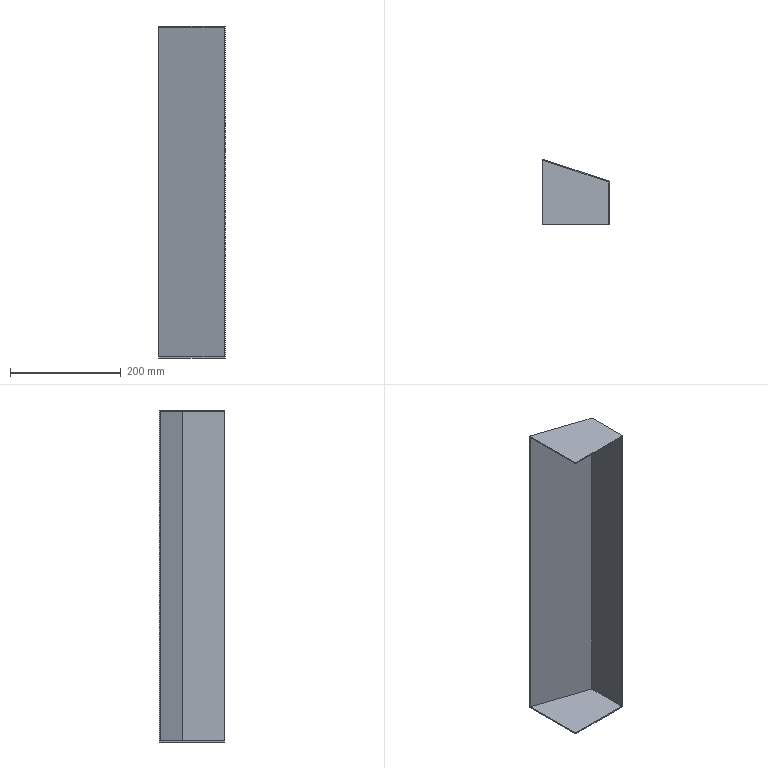Part | SolidWorks | features Extrusion 1, ICE 1, Shell 1 | 1 solid | 10 faces | box 120 x 118 x 600 mm | volume 288678 mm3 | plane 10
STEP:
#1=CARTESIAN_POINT('',(0.,120.,-300.));
#2=VERTEX_POINT('',#1);
#3=CARTESIAN_POINT('',(0.,2.,-300.));
#4=VERTEX_POINT('',#3);
#5=CARTESIAN_POINT('',(0.,0.,-300.));
#6=DIRECTION('',(0.,-1.,0.));
#7=VECTOR('',#6,1000.);
#8=LINE('',#5,#7);
#9=EDGE_CURVE('',#2,#4,#8,.T.);
#10=ORIENTED_EDGE('',*,*,#9,.T.);
#11=CARTESIAN_POINT('',(0.,2.,-298.));
#12=VERTEX_POINT('',#11);
#13=CARTESIAN_POINT('',(0.,2.,300.));
#14=DIRECTION('',(0.,0.,-1.));
#15=VECTOR('',#14,1000.);
#16=LINE('',#13,#15);
#17=EDGE_CURVE('',#12,#4,#16,.T.);
#18=ORIENTED_EDGE('',*,*,#17,.F.);
#19=CARTESIAN_POINT('',(0.,117.892,-298.));
#20=VERTEX_POINT('',#19);
#21=CARTESIAN_POINT('',(0.,0.,-298.));
#22=DIRECTION('',(0.,-1.,0.));
#23=VECTOR('',#22,1000.);
#24=LINE('',#21,#23);
#25=EDGE_CURVE('',#20,#12,#24,.T.);
#26=ORIENTED_EDGE('',*,*,#25,.F.);
#27=CARTESIAN_POINT('',(0.,117.892,298.));
#28=VERTEX_POINT('',#27);
#29=CARTESIAN_POINT('',(0.,117.892,300.));
#30=DIRECTION('',(0.,0.,-1.));
#31=VECTOR('',#30,1000.);
#32=LINE('',#29,#31);
#33=EDGE_CURVE('',#28,#20,#32,.T.);
#34=ORIENTED_EDGE('',*,*,#33,.F.);
#35=CARTESIAN_POINT('',(0.,2.,298.));
#36=VERTEX_POINT('',#35);
#37=CARTESIAN_POINT('',(0.,0.,298.));
#38=DIRECTION('',(0.,-1.,0.));
#39=VECTOR('',#38,1000.);
#40=LINE('',#37,#39);
#41=EDGE_CURVE('',#28,#36,#40,.T.);
#42=ORIENTED_EDGE('',*,*,#41,.T.);
#43=CARTESIAN_POINT('',(0.,2.,300.));
#44=VERTEX_POINT('',#43);
#45=CARTESIAN_POINT('',(0.,2.,300.));
#46=DIRECTION('',(0.,0.,-1.));
#47=VECTOR('',#46,1000.);
#48=LINE('',#45,#47);
#49=EDGE_CURVE('',#44,#36,#48,.T.);
#50=ORIENTED_EDGE('',*,*,#49,.F.);
#51=CARTESIAN_POINT('',(0.,120.,300.));
#52=VERTEX_POINT('',#51);
#53=CARTESIAN_POINT('',(0.,0.,300.));
#54=DIRECTION('',(0.,-1.,0.));
#55=VECTOR('',#54,1000.);
#56=LINE('',#53,#55);
#57=EDGE_CURVE('',#52,#44,#56,.T.);
#58=ORIENTED_EDGE('',*,*,#57,.F.);
#59=CARTESIAN_POINT('',(0.,120.,300.));
#60=DIRECTION('',(0.,0.,-1.));
#61=VECTOR('',#60,1000.);
#62=LINE('',#59,#61);
#63=EDGE_CURVE('',#52,#2,#62,.T.);
#64=ORIENTED_EDGE('',*,*,#63,.T.);
#65=EDGE_LOOP('',(#10,#18,#26,#34,#42,#50,#58,#64));
#66=FACE_OUTER_BOUND('',#65,.T.);
#67=CARTESIAN_POINT('',(0.,0.,300.));
#68=DIRECTION('',(1.,0.,0.));
#69=DIRECTION('',(0.,0.,-1.));
#70=AXIS2_PLACEMENT_3D('',#67,#68,#69);
#71=PLANE('',#70);
#72=ADVANCED_FACE('',(#66),#71,.F.);
#73=CARTESIAN_POINT('',(120.,2.,300.));
#74=VERTEX_POINT('',#73);
#75=CARTESIAN_POINT('',(120.,80.,300.));
#76=VERTEX_POINT('',#75);
#77=CARTESIAN_POINT('',(120.,80.,300.));
#78=DIRECTION('',(0.,1.,0.));
#79=VECTOR('',#78,1000.);
#80=LINE('',#77,#79);
#81=EDGE_CURVE('',#74,#76,#80,.T.);
#82=ORIENTED_EDGE('',*,*,#81,.F.);
#83=CARTESIAN_POINT('',(120.,2.,-300.));
#84=VERTEX_POINT('',#83);
#85=CARTESIAN_POINT('',(120.,2.,300.));
#86=DIRECTION('',(0.,0.,1.));
#87=VECTOR('',#86,1000.);
#88=LINE('',#85,#87);
#89=EDGE_CURVE('',#84,#74,#88,.T.);
#90=ORIENTED_EDGE('',*,*,#89,.F.);
#91=CARTESIAN_POINT('',(120.,80.,-300.));
#92=VERTEX_POINT('',#91);
#93=CARTESIAN_POINT('',(120.,80.,-300.));
#94=DIRECTION('',(0.,1.,0.));
#95=VECTOR('',#94,1000.);
#96=LINE('',#93,#95);
#97=EDGE_CURVE('',#84,#92,#96,.T.);
#98=ORIENTED_EDGE('',*,*,#97,.T.);
#99=CARTESIAN_POINT('',(120.,80.,300.));
#100=DIRECTION('',(0.,0.,-1.));
#101=VECTOR('',#100,1000.);
#102=LINE('',#99,#101);
#103=EDGE_CURVE('',#76,#92,#102,.T.);
#104=ORIENTED_EDGE('',*,*,#103,.F.);
#105=EDGE_LOOP('',(#82,#90,#98,#104));
#106=FACE_OUTER_BOUND('',#105,.T.);
#107=CARTESIAN_POINT('',(120.,80.,300.));
#108=DIRECTION('',(-1.,0.,0.));
#109=DIRECTION('',(0.,0.,1.));
#110=AXIS2_PLACEMENT_3D('',#107,#108,#109);
#111=PLANE('',#110);
#112=ADVANCED_FACE('',(#106),#111,.F.);
#113=CARTESIAN_POINT('',(0.,120.,-300.));
#114=DIRECTION('',(-0.9487,0.3162,0.));
#115=VECTOR('',#114,1000.);
#116=LINE('',#113,#115);
#117=EDGE_CURVE('',#92,#2,#116,.T.);
#118=ORIENTED_EDGE('',*,*,#117,.T.);
#119=ORIENTED_EDGE('',*,*,#63,.F.);
#120=CARTESIAN_POINT('',(0.,120.,300.));
#121=DIRECTION('',(-0.9487,0.3162,0.));
#122=VECTOR('',#121,1000.);
#123=LINE('',#120,#122);
#124=EDGE_CURVE('',#76,#52,#123,.T.);
#125=ORIENTED_EDGE('',*,*,#124,.F.);
#126=ORIENTED_EDGE('',*,*,#103,.T.);
#127=EDGE_LOOP('',(#118,#119,#125,#126));
#128=FACE_OUTER_BOUND('',#127,.T.);
#129=CARTESIAN_POINT('',(0.,120.,300.));
#130=DIRECTION('',(-0.3162,-0.9487,0.));
#131=DIRECTION('',(0.9487,-0.3162,0.));
#132=AXIS2_PLACEMENT_3D('',#129,#130,#131);
#133=PLANE('',#132);
#134=ADVANCED_FACE('',(#128),#133,.F.);
#135=CARTESIAN_POINT('',(120.,2.,300.));
#136=DIRECTION('',(-1.,0.,0.));
#137=VECTOR('',#136,1000.);
#138=LINE('',#135,#137);
#139=EDGE_CURVE('',#74,#44,#138,.T.);
#140=ORIENTED_EDGE('',*,*,#139,.F.);
#141=ORIENTED_EDGE('',*,*,#81,.T.);
#142=ORIENTED_EDGE('',*,*,#124,.T.);
#143=ORIENTED_EDGE('',*,*,#57,.T.);
#144=EDGE_LOOP('',(#140,#141,#142,#143));
#145=FACE_OUTER_BOUND('',#144,.T.);
#146=CARTESIAN_POINT('',(0.,0.,300.));
#147=DIRECTION('',(0.,0.,1.));
#148=DIRECTION('',(1.,0.,0.));
#149=AXIS2_PLACEMENT_3D('',#146,#147,#148);
#150=PLANE('',#149);
#151=ADVANCED_FACE('',(#145),#150,.T.);
#152=ORIENTED_EDGE('',*,*,#97,.F.);
#153=CARTESIAN_POINT('',(120.,2.,-300.));
#154=DIRECTION('',(1.,0.,0.));
#155=VECTOR('',#154,1000.);
#156=LINE('',#153,#155);
#157=EDGE_CURVE('',#4,#84,#156,.T.);
#158=ORIENTED_EDGE('',*,*,#157,.F.);
#159=ORIENTED_EDGE('',*,*,#9,.F.);
#160=ORIENTED_EDGE('',*,*,#117,.F.);
#161=EDGE_LOOP('',(#152,#158,#159,#160));
#162=FACE_OUTER_BOUND('',#161,.T.);
#163=CARTESIAN_POINT('',(0.,0.,-300.));
#164=DIRECTION('',(0.,0.,1.));
#165=DIRECTION('',(1.,0.,0.));
#166=AXIS2_PLACEMENT_3D('',#163,#164,#165);
#167=PLANE('',#166);
#168=ADVANCED_FACE('',(#162),#167,.F.);
#169=CARTESIAN_POINT('',(118.,2.,-298.));
#170=VERTEX_POINT('',#169);
#171=CARTESIAN_POINT('',(118.,78.558,-298.));
#172=VERTEX_POINT('',#171);
#173=CARTESIAN_POINT('',(118.,80.,-298.));
#174=DIRECTION('',(0.,1.,0.));
#175=VECTOR('',#174,1000.);
#176=LINE('',#173,#175);
#177=EDGE_CURVE('',#170,#172,#176,.T.);
#178=ORIENTED_EDGE('',*,*,#177,.F.);
#179=CARTESIAN_POINT('',(118.,2.,298.));
#180=VERTEX_POINT('',#179);
#181=CARTESIAN_POINT('',(118.,2.,300.));
#182=DIRECTION('',(0.,0.,-1.));
#183=VECTOR('',#182,1000.);
#184=LINE('',#181,#183);
#185=EDGE_CURVE('',#180,#170,#184,.T.);
#186=ORIENTED_EDGE('',*,*,#185,.F.);
#187=CARTESIAN_POINT('',(118.,78.558,298.));
#188=VERTEX_POINT('',#187);
#189=CARTESIAN_POINT('',(118.,80.,298.));
#190=DIRECTION('',(0.,1.,0.));
#191=VECTOR('',#190,1000.);
#192=LINE('',#189,#191);
#193=EDGE_CURVE('',#180,#188,#192,.T.);
#194=ORIENTED_EDGE('',*,*,#193,.T.);
#195=CARTESIAN_POINT('',(118.,78.558,300.));
#196=DIRECTION('',(0.,0.,-1.));
#197=VECTOR('',#196,1000.);
#198=LINE('',#195,#197);
#199=EDGE_CURVE('',#188,#172,#198,.T.);
#200=ORIENTED_EDGE('',*,*,#199,.T.);
#201=EDGE_LOOP('',(#178,#186,#194,#200));
#202=FACE_OUTER_BOUND('',#201,.T.);
#203=CARTESIAN_POINT('',(118.,80.,300.));
#204=DIRECTION('',(-1.,0.,0.));
#205=DIRECTION('',(0.,0.,1.));
#206=AXIS2_PLACEMENT_3D('',#203,#204,#205);
#207=PLANE('',#206);
#208=ADVANCED_FACE('',(#202),#207,.T.);
#209=CARTESIAN_POINT('',(-0.6325,118.103,-298.));
#210=DIRECTION('',(-0.9487,0.3162,0.));
#211=VECTOR('',#210,1000.);
#212=LINE('',#209,#211);
#213=EDGE_CURVE('',#172,#20,#212,.T.);
#214=ORIENTED_EDGE('',*,*,#213,.F.);
#215=ORIENTED_EDGE('',*,*,#199,.F.);
#216=CARTESIAN_POINT('',(-0.6325,118.103,298.));
#217=DIRECTION('',(-0.9487,0.3162,0.));
#218=VECTOR('',#217,1000.);
#219=LINE('',#216,#218);
#220=EDGE_CURVE('',#188,#28,#219,.T.);
#221=ORIENTED_EDGE('',*,*,#220,.T.);
#222=ORIENTED_EDGE('',*,*,#33,.T.);
#223=EDGE_LOOP('',(#214,#215,#221,#222));
#224=FACE_OUTER_BOUND('',#223,.T.);
#225=CARTESIAN_POINT('',(-0.6325,118.103,300.));
#226=DIRECTION('',(-0.3162,-0.9487,0.));
#227=DIRECTION('',(0.9487,-0.3162,0.));
#228=AXIS2_PLACEMENT_3D('',#225,#226,#227);
#229=PLANE('',#228);
#230=ADVANCED_FACE('',(#224),#229,.T.);
#231=ORIENTED_EDGE('',*,*,#41,.F.);
#232=ORIENTED_EDGE('',*,*,#220,.F.);
#233=ORIENTED_EDGE('',*,*,#193,.F.);
#234=CARTESIAN_POINT('',(120.,2.,298.));
#235=DIRECTION('',(1.,0.,0.));
#236=VECTOR('',#235,1000.);
#237=LINE('',#234,#236);
#238=EDGE_CURVE('',#36,#180,#237,.T.);
#239=ORIENTED_EDGE('',*,*,#238,.F.);
#240=EDGE_LOOP('',(#231,#232,#233,#239));
#241=FACE_OUTER_BOUND('',#240,.T.);
#242=CARTESIAN_POINT('',(0.,0.,298.));
#243=DIRECTION('',(0.,0.,1.));
#244=DIRECTION('',(1.,0.,0.));
#245=AXIS2_PLACEMENT_3D('',#242,#243,#244);
#246=PLANE('',#245);
#247=ADVANCED_FACE('',(#241),#246,.F.);
#248=ORIENTED_EDGE('',*,*,#25,.T.);
#249=CARTESIAN_POINT('',(120.,2.,-298.));
#250=DIRECTION('',(1.,0.,0.));
#251=VECTOR('',#250,1000.);
#252=LINE('',#249,#251);
#253=EDGE_CURVE('',#12,#170,#252,.T.);
#254=ORIENTED_EDGE('',*,*,#253,.T.);
#255=ORIENTED_EDGE('',*,*,#177,.T.);
#256=ORIENTED_EDGE('',*,*,#213,.T.);
#257=EDGE_LOOP('',(#248,#254,#255,#256));
#258=FACE_OUTER_BOUND('',#257,.T.);
#259=CARTESIAN_POINT('',(0.,0.,-298.));
#260=DIRECTION('',(0.,0.,1.));
#261=DIRECTION('',(1.,0.,0.));
#262=AXIS2_PLACEMENT_3D('',#259,#260,#261);
#263=PLANE('',#262);
#264=ADVANCED_FACE('',(#258),#263,.T.);
#265=ORIENTED_EDGE('',*,*,#185,.T.);
#266=ORIENTED_EDGE('',*,*,#253,.F.);
#267=ORIENTED_EDGE('',*,*,#17,.T.);
#268=ORIENTED_EDGE('',*,*,#157,.T.);
#269=ORIENTED_EDGE('',*,*,#89,.T.);
#270=ORIENTED_EDGE('',*,*,#139,.T.);
#271=ORIENTED_EDGE('',*,*,#49,.T.);
#272=ORIENTED_EDGE('',*,*,#238,.T.);
#273=EDGE_LOOP('',(#265,#266,#267,#268,#269,#270,#271,#272));
#274=FACE_OUTER_BOUND('',#273,.T.);
#275=CARTESIAN_POINT('',(120.,2.,300.));
#276=DIRECTION('',(0.,1.,0.));
#277=DIRECTION('',(0.,0.,1.));
#278=AXIS2_PLACEMENT_3D('',#275,#276,#277);
#279=PLANE('',#278);
#280=ADVANCED_FACE('',(#274),#279,.F.);
#281=CLOSED_SHELL('',(#72,#112,#134,#151,#168,#208,#230,#247,#264,#280));
#282=MANIFOLD_SOLID_BREP('',#281);
#283=CARTESIAN_POINT('',(0.,0.,0.));
#284=DIRECTION('',(0.,0.,1.));
#285=DIRECTION('',(1.,0.,0.));
#286=AXIS2_PLACEMENT_3D('',#283,#284,#285);
#287=(LENGTH_UNIT()NAMED_UNIT(*)SI_UNIT(.MILLI.,.METRE.));
#288=UNCERTAINTY_MEASURE_WITH_UNIT(LENGTH_MEASURE(0.00001),#287,'','');
#289=(NAMED_UNIT(*)PLANE_ANGLE_UNIT()SI_UNIT($,.RADIAN.));
#290=(NAMED_UNIT(*)SI_UNIT($,.STERADIAN.)SOLID_ANGLE_UNIT());
#291=(GEOMETRIC_REPRESENTATION_CONTEXT(3)GLOBAL_UNCERTAINTY_ASSIGNED_CONTEXT((#288))GLOBAL_UNIT_ASSIGNED_CONTEXT((#287,#289,#290))REPRESENTATION_CONTEXT('',''));
#292=ADVANCED_BREP_SHAPE_REPRESENTATION('',(#282,#286),#291);